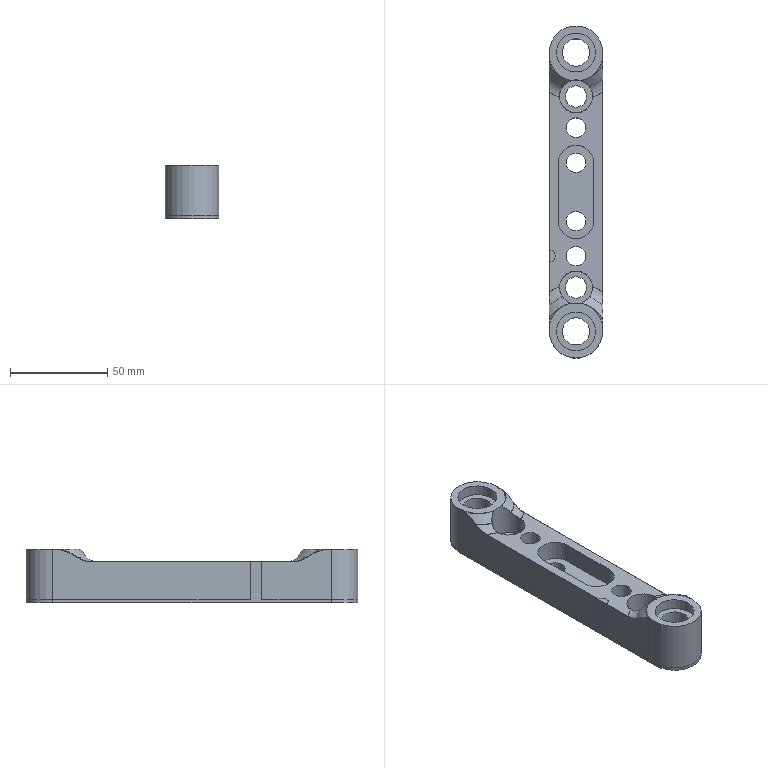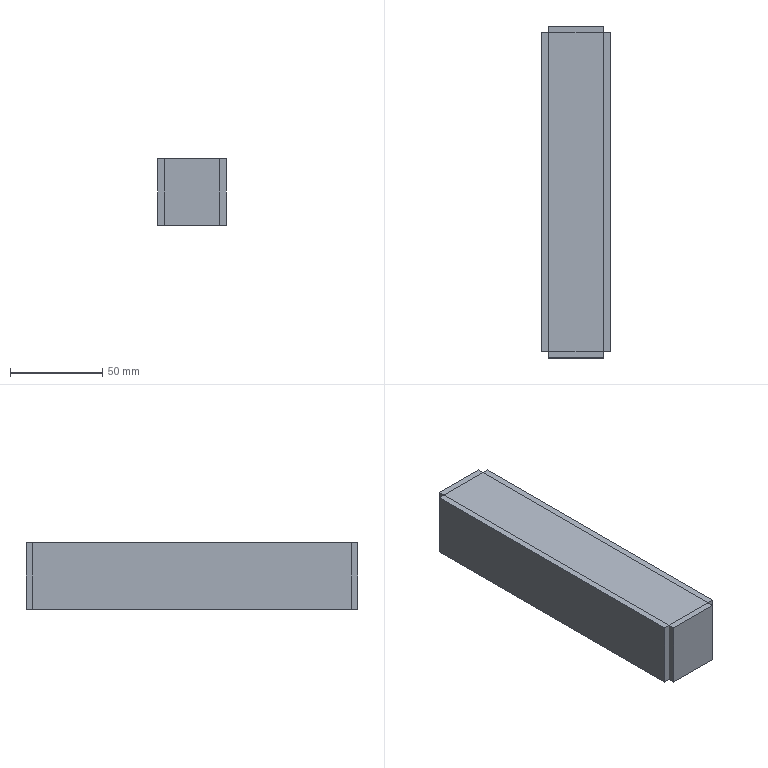CAM job | NX | 3-axis milling, 5-axis milling, drilling | part box 27.4 x 170.48 x 27.5 mm | stock box 36.92 x 180 x 36 mm
Tools:
number,name,description,diameter,corner_radius,flute_length,length,flutes
2,D8点钻,定心钻D8,8.0,0.0,75.0,117.0,2
6,D8开粗,D8,8.0,0.0,20.0,60.0,2
8,D8精光,D8,8.0,0.0,20.0,60.0,2
5,D12开粗,D12,12.0,0.0,30.0,75.0,2
7,D12精光,D12,12.0,0.0,30.0,75.0,2
9,D3倒角刀,DJ4-32,3.0,0.0,1.5,50.0,2
11,D6倒角刀,DJ6-32,6.0,0.0,3.0,50.0,2
10,R3,球头铣刀,6.0,3.0,12.0,50.0,2
17,Z8.5,Z8.5直柄钻头,8.5,0.0,75.0,117.0,2
18,M10X1.5,公制-铝用螺旋槽丝攻,8.6,0.0,24.0,27.0,2
1,D50R0.8,Milling Tool-5 Parameters,50.0,0.8,50.0,75.0,2
3,D9.5钻头,Drilling Tool,9.5,0.0,35.0,50.0,2
4,D11钻头,Drilling Tool,11.0,0.0,35.0,50.0,2
12,D14钻头,Drilling Tool,14.0,0.0,35.0,50.0,2
13,D10镗刀,Drilling Tool,10.0,0.0,35.0,50.0,2
14,D20镗刀,Drilling Tool,20.0,0.0,35.0,50.0,2
15,M16螺纹铣刀,Thread Mill,9.9,0.0,32.0,50.0,32
0,D5开粗,Milling Tool-5 Parameters,5.0,0.0,50.0,75.0,2
0,M10螺纹铣刀,Thread Mill,8.2,0.0,10.0,50.0,3
Operations:
program,operation,operation_type,tool,method,geometry_group,spindle_rpm,surface_speed,feed_per_tooth,feed_cut,feed_plunge,cut_length_mm,path_length_mm,cut_time_min,machine_time_min
XX-CNC1,PLANAR_MILL,PlanarMilling,D50R0.8,METHOD,W1,2000.0,100.0,0.1178,800.0,100.0,244.0,298.8,0.305,0.3105
XX-CNC1,PLANAR_MILL_COPY_1,PlanarMilling,D50R0.8,METHOD,W1,2000.0,100.0,0.1178,800.0,100.0,244.0,299.4,0.305,0.3105
XX-CNC1,DRILLING,Operation,D8点钻,METHOD,MCS_1,2500.0,0.0,0.0,200.0,0.0,36.0,297.681,0.18,0.2062
XX-CNC1,DRILLING_COPY,Operation,D9.5钻头,METHOD,MCS_1,1600.0,0.0,0.0,150.0,0.0,76.0,281.068,0.5067,0.5272
XX-CNC1,DRILLING_COPY_COPY_1,Operation,Z8.5,METHOD,MCS_1,1600.0,0.0,0.0,150.0,0.0,76.0,245.15,0.5067,0.5236
XX-CNC1,DRILLING_COPY_COPY,Operation,D11钻头,METHOD,MCS_1,1600.0,0.0,0.0,150.0,0.0,152.0,516.523,1.013,1.05
XX-CNC1,ADAPTIVE_MILLING,CavityMilling,D12开粗,METHOD,W1,4000.0,100.0,0.1178,1500.0,100.0,21296.969,24097.413,9.392,9.672
XX-CNC1,ADAPTIVE_MILLING_COPY,CavityMilling,D8开粗,METHOD,W1,4000.0,100.0,0.1178,1500.0,100.0,10341.181,11927.931,6.213,6.372
XX-CNC1,PLANAR_MILL_11,PlanarMilling,D8开粗,METHOD,MCS_1,3500.0,87.0,0.1143,800.0,100.0,1870.744,2179.284,2.338,2.369
XX-CNC1,PLANAR_MILL_1,PlanarMilling,D12精光,METHOD,W1,3500.0,100.0,0.1178,800.0,100.0,842.957,960.957,1.054,1.065
XX-CNC1,PLANAR_MILL_2,PlanarMilling,D8开粗,METHOD,W1,3500.0,100.0,0.0714,500.0,100.0,150.224,428.229,0.3004,0.3282
XX-CNC1,PLANAR_MILL_3,PlanarMilling,D3倒角刀,METHOD,W1,3500.0,100.0,0.1178,800.0,100.0,117.558,370.637,0.1469,0.1723
XX-CNC1,PLANAR_MILL_3_COPY,PlanarMilling,D3倒角刀,METHOD,W1,3500.0,100.0,0.1178,800.0,100.0,226.285,401.885,0.2829,0.3004
XX-CNC1,PLANAR_MILL_3_COPY_COPY,PlanarMilling,D3倒角刀,METHOD,W1,3500.0,100.0,0.1178,800.0,100.0,133.592,393.28,0.167,0.193
XX-CNC1,PLANAR_MILL_3_COPY_COPY_COPY,PlanarMilling,D3倒角刀,METHOD,W1,3500.0,32.0,0.1143,800.0,100.0,81.115,359.115,0.1014,0.1292
XX-CNC2,ADAPTIVE_MILLING_1,CavityMilling,D12开粗,METHOD,W2,4000.0,100.0,0.1178,1500.0,100.0,11010.587,11064.288,7.336,7.341
XX-CNC2,PLANAR_MILL_10_COPY_1,PlanarMilling,D8开粗,METHOD,MCS_2,3500.0,87.0,0.1143,800.0,100.0,242.772,498.993,0.3035,0.3291
XX-CNC2,PLANAR_MILL_10,PlanarMilling,D8开粗,METHOD,MCS_2,3500.0,87.0,0.1143,800.0,100.0,568.881,843.296,0.7111,0.7385
XX-CNC2,PLANAR_MILL_10_COPY,PlanarMilling,D8开粗,METHOD,MCS_2,3500.0,87.0,0.0571,400.0,100.0,74.761,373.846,0.1869,0.2168
XX-CNC2,PLANAR_MILL_4,PlanarMilling,D50R0.8,METHOD,W2,2000.0,100.0,0.1178,600.0,100.0,228.48,284.44,0.3808,0.3864
XX-CNC2,THREAD_MILLING_1,ThreadMilling,M10螺纹铣刀,METHOD,MCS_2,3000.0,0.0,0.0,250.0,100.0,342.007,713.675,1.368,1.405
XX-CNC2,PLANAR_MILL_5,PlanarMilling,D6倒角刀,METHOD,W2,3500.0,100.0,0.1178,800.0,100.0,386.921,446.921,0.4837,0.4897
XX-CNC2,PLANAR_MILL_5_COPY,PlanarMilling,D6倒角刀,METHOD,W2,3500.0,100.0,0.1178,800.0,100.0,385.664,445.664,0.4821,0.4881
XX-CNC2,PLANAR_MILL_6,PlanarMilling,D6倒角刀,METHOD,W2,3500.0,65.0,0.0571,400.0,100.0,102.072,365.29,0.2552,0.2815
XX-CNC2,PLANAR_MILL_6_COPY,PlanarMilling,D6倒角刀,METHOD,W2,3500.0,100.0,0.1178,800.0,100.0,139.123,469.583,0.1739,0.207
XX-CNC2,PLANAR_MILL_6_COPY_COPY,PlanarMilling,D6倒角刀,METHOD,W2,3500.0,100.0,0.1178,800.0,100.0,55.457,207.457,0.0693,0.0845
XX-CNC2,PLANAR_MILL_4_COPY,PlanarMilling,D50R0.8,METHOD,W2,2000.0,100.0,0.1178,600.0,100.0,228.48,284.48,0.3808,0.3864
XX-CNC3,PLANAR_MILL_COPY,PlanarMilling,D50R0.8,METHOD,W1,2000.0,100.0,0.1178,800.0,100.0,244.0,299.9,0.305,0.3106
XX-CNC3,PLANAR_MILL_COPY_COPY,PlanarMilling,D50R0.8,METHOD,W1,2000.0,100.0,0.1178,800.0,100.0,244.0,300.0,0.305,0.3106
XX-CNC3,FLOOR_FACING_COPY,VolumeBased25DMillingOperation,D12开粗,METHOD,MCS_1,3000.0,100.0,0.1178,800.0,100.0,400.92,467.72,0.5012,0.5078
XX-CNC3,PLANAR_MILL_8_COPY,PlanarMilling,D12开粗,METHOD,MCS_1,3000.0,100.0,0.1178,800.0,100.0,92.948,321.939,0.1162,0.1391
XX-CNC3,PLANAR_MILL_1_COPY,PlanarMilling,D12精光,METHOD,W1,3000.0,100.0,0.1178,800.0,100.0,841.174,952.174,1.052,1.063
XX-CNC3,FLOOR_FACING,VolumeBased25DMillingOperation,D12精光,METHOD,MCS_1,3000.0,100.0,0.1178,800.0,100.0,391.784,458.784,0.4897,0.4964
XX-CNC3,PLANAR_MILL_8,PlanarMilling,D12精光,METHOD,MCS_1,3000.0,100.0,0.1178,800.0,100.0,92.948,322.339,0.1162,0.1391
XX-CNC3,PLANAR_MILL_9_COPY_1,PlanarMilling,D8精光,METHOD,MCS_1,3000.0,100.0,0.1178,800.0,100.0,170.554,259.354,0.2132,0.2221
XX-CNC3,PLANAR_MILL_9,PlanarMilling,D8精光,METHOD,MCS_1,3000.0,100.0,0.1178,800.0,100.0,171.811,260.811,0.2148,0.2237
XX-CNC3,PLANAR_MILL_9_COPY,PlanarMilling,D8精光,METHOD,MCS_1,3000.0,100.0,0.1178,800.0,100.0,210.94,299.94,0.2637,0.2726
XX-CNC3,PLANAR_MILL_13_COPY_1,PlanarMilling,D8开粗,METHOD,MCS_1,3000.0,100.0,0.1178,600.0,100.0,198.292,475.431,0.3305,0.3582
XX-CNC3,PLANAR_MILL_13,PlanarMilling,D8开粗,METHOD,MCS_1,3000.0,100.0,0.1178,600.0,100.0,82.285,625.946,0.1371,0.1915
XX-CNC3,CURVE_DRIVE,SurfaceContour,R3,METHOD,MCS_1,4000.0,50.0,0.1875,1500.0,100.0,8799.105,9237.429,5.866,5.91
XX-CNC3,3_AXIS_DEBURRING,TpMultiAxisDeburring,R3,METHOD,MCS_1,3500.0,0.0,0.0,800.0,90.0,542.308,582.671,0.6803,0.6803
XX-CNC3,DRILLING_1,Operation,D14钻头,METHOD,MCS_1,800.0,0.0,0.0,100.0,0.0,63.0,332.111,0.63,0.6569
XX-CNC3,DRILLING_2,Operation,D10镗刀,METHOD,MCS_1,800.0,0.0,0.0,60.0,0.0,52.0,246.068,0.8667,0.8861
XX-CNC3,DRILLING_3,Operation,D20镗刀,METHOD,MCS_1,800.0,0.0,0.0,60.0,0.0,17.0,240.111,0.2833,0.3056
XX-CNC3,PLANAR_MILL_3_COPY_COPY_COPY_1_COPY,PlanarMilling,D6倒角刀,METHOD,W1,3500.0,100.0,0.1178,800.0,100.0,95.727,386.007,0.1197,0.1487
XX-CNC3,PLANAR_MILL_3_COPY_COPY_COPY_1_COPY_COPY_1,PlanarMilling,D6倒角刀,METHOD,W1,3500.0,100.0,0.1178,800.0,100.0,55.457,273.457,0.0693,0.0911
XX-CNC3,THREAD_MILLING,ThreadMilling,M16螺纹铣刀,METHOD,MCS_1,3000.0,93.0,0.0036,300.0,100.0,1727.516,2503.683,5.758,5.836
XX-CNC3,PLANAR_MILL_14,PlanarMilling,D5开粗,METHOD,MCS_1,3500.0,43.0,0.0857,600.0,100.0,1400.846,1593.366,2.335,2.354
XX-CNC3,PLANAR_MILL_3_COPY_1,PlanarMilling,D3倒角刀,METHOD,W1,3500.0,100.0,0.1178,800.0,100.0,116.929,370.009,0.1462,0.1715
XX-CNC3,PLANAR_MILL_3_COPY_COPY_COPY_1,PlanarMilling,D3倒角刀,METHOD,W1,3500.0,100.0,0.1178,800.0,100.0,134.831,394.538,0.1685,0.1945
XX-CNC3,PLANAR_MILL_3_COPY_COPY_COPY_1_COPY_COPY_COPY,PlanarMilling,D3倒角刀,METHOD,W1,3500.0,100.0,0.1178,800.0,100.0,13.425,84.425,0.0168,0.0239
XX-CNC3,PLANAR_MILL_3_COPY_COPY_COPY_1_COPY_COPY,PlanarMilling,D3倒角刀,METHOD,W1,3500.0,100.0,0.1178,800.0,100.0,182.642,471.017,0.2283,0.2571
XX-CNC5,DRILLING_4,Operation,D8点钻,METHOD,MCS_5,2000.0,0.0,0.0,200.0,0.0,18.0,248.523,0.09,0.1131
XX-CNC5,DRILLING_5_COPY_1_COPY,Operation,D8点钻,METHOD,MCS_5,2000.0,0.0,0.0,200.0,0.0,18.0,171.646,0.09,0.1054
XX-CNC5,DRILLING_5_COPY_1,Operation,Z8.5,METHOD,MCS_5,2000.0,0.0,0.0,200.0,0.0,36.0,207.646,0.18,0.1972
XX-CNC5,DRILLING_5,Operation,Z8.5,METHOD,MCS_5,2000.0,0.0,0.0,200.0,0.0,32.0,270.111,0.16,0.1838
XX-CNC5,DRILLING_5_COPY,Operation,Z8.5,METHOD,MCS_5,2000.0,0.0,0.0,200.0,0.0,56.0,273.046,0.28,0.3017
XX-CNC5,PLANAR_MILL_7,PlanarMilling,D8点钻,METHOD,MCS_5,3000.0,75.0,0.1,600.0,100.0,149.24,533.688,0.2487,0.2872
XX-CNC5,DRILLING_5_COPY_COPY,Operation,M10X1.5,METHOD,MCS_5,300.0,8.0,0.0025,1.5,0.0,26.0,213.046,17.333,17.352
XX-CNC5,PLANAR_MILL_12,PlanarMilling,D8开粗,METHOD,MCS_5,3000.0,75.0,0.1,600.0,100.0,1286.447,1563.814,2.144,2.172
XX-CNC5,PLANAR_MILL_12_COPY,PlanarMilling,D8开粗,METHOD,MCS_5,3000.0,75.0,0.1,400.0,100.0,74.761,368.503,0.1869,0.2163